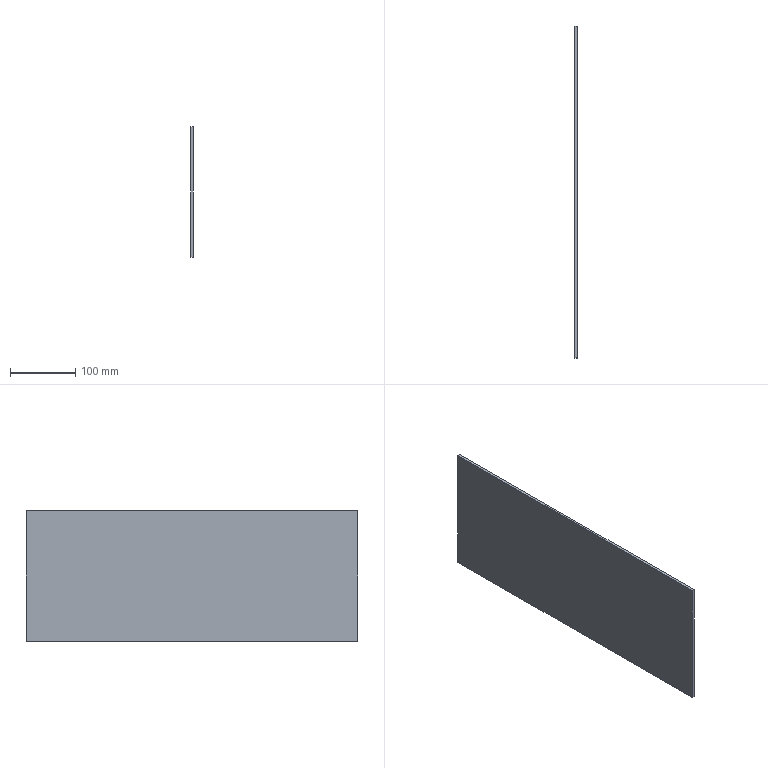Part | STEP file | 1 solid | 6 faces | box 4 x 509.4 x 200.9 mm | volume 409354 mm3 | plane 6
STEP:
#1=CARTESIAN_POINT('',(0.,0.,0.));
#2=DIRECTION('',(0.,0.,1.));
#3=DIRECTION('',(1.,0.,0.));
#4=AXIS2_PLACEMENT_3D('',#1,#2,#3);
#5=CARTESIAN_POINT('',(761.,3906.,1648.194));
#6=VERTEX_POINT('',#5);
#7=CARTESIAN_POINT('',(761.,3906.,1447.294));
#8=VERTEX_POINT('',#7);
#9=CARTESIAN_POINT('',(761.,3906.,1648.194));
#10=DIRECTION('',(0.,0.,-1.));
#11=VECTOR('',#10,1.);
#12=LINE('',#9,#11);
#13=CARTESIAN_POINT('',(765.,3906.,1447.294));
#14=DIRECTION('',(0.,-1.,0.));
#15=DIRECTION('',(0.,0.,-1.));
#16=AXIS2_PLACEMENT_3D('',#13,#14,#15);
#17=PLANE('',#16);
#18=CARTESIAN_POINT('',(-200.9,-4.));
#19=DIRECTION('',(1.,0.));
#20=VECTOR('',#19,1.);
#21=LINE('',#18,#20);
#22=(GEOMETRIC_REPRESENTATION_CONTEXT(2)PARAMETRIC_REPRESENTATION_CONTEXT()REPRESENTATION_CONTEXT('',''));
#23=DEFINITIONAL_REPRESENTATION('',(#21),#22);
#24=PCURVE('',#17,#23);
#25=CARTESIAN_POINT('',(761.,0.,0.));
#26=DIRECTION('',(-1.,0.,0.));
#27=DIRECTION('',(0.,0.,1.));
#28=AXIS2_PLACEMENT_3D('',#25,#26,#27);
#29=PLANE('',#28);
#30=CARTESIAN_POINT('',(1648.194,3906.));
#31=DIRECTION('',(-1.,0.));
#32=VECTOR('',#31,1.);
#33=LINE('',#30,#32);
#34=(GEOMETRIC_REPRESENTATION_CONTEXT(2)PARAMETRIC_REPRESENTATION_CONTEXT()REPRESENTATION_CONTEXT('',''));
#35=DEFINITIONAL_REPRESENTATION('',(#33),#34);
#36=PCURVE('',#29,#35);
#37=SURFACE_CURVE('',#12,(#24,#36),.PCURVE_S1.);
#38=EDGE_CURVE('',#6,#8,#37,.T.);
#39=ORIENTED_EDGE('',*,*,#38,.F.);
#40=CARTESIAN_POINT('',(765.,3906.,1648.194));
#41=VERTEX_POINT('',#40);
#42=CARTESIAN_POINT('',(761.,3906.,1648.194));
#43=DIRECTION('',(1.,0.,0.));
#44=VECTOR('',#43,1.);
#45=LINE('',#42,#44);
#46=CARTESIAN_POINT('',(-200.9,-4.));
#47=DIRECTION('',(0.,1.));
#48=VECTOR('',#47,1.);
#49=LINE('',#46,#48);
#50=(GEOMETRIC_REPRESENTATION_CONTEXT(2)PARAMETRIC_REPRESENTATION_CONTEXT()REPRESENTATION_CONTEXT('',''));
#51=DEFINITIONAL_REPRESENTATION('',(#49),#50);
#52=PCURVE('',#17,#51);
#53=CARTESIAN_POINT('',(765.,3906.,1648.194));
#54=DIRECTION('',(0.,0.,1.));
#55=DIRECTION('',(1.,0.,0.));
#56=AXIS2_PLACEMENT_3D('',#53,#54,#55);
#57=PLANE('',#56);
#58=CARTESIAN_POINT('',(-4.,0.));
#59=DIRECTION('',(1.,0.));
#60=VECTOR('',#59,1.);
#61=LINE('',#58,#60);
#62=(GEOMETRIC_REPRESENTATION_CONTEXT(2)PARAMETRIC_REPRESENTATION_CONTEXT()REPRESENTATION_CONTEXT('',''));
#63=DEFINITIONAL_REPRESENTATION('',(#61),#62);
#64=PCURVE('',#57,#63);
#65=SURFACE_CURVE('',#45,(#52,#64),.PCURVE_S1.);
#66=EDGE_CURVE('',#6,#41,#65,.T.);
#67=ORIENTED_EDGE('',*,*,#66,.T.);
#68=CARTESIAN_POINT('',(765.,3906.,1447.294));
#69=VERTEX_POINT('',#68);
#70=CARTESIAN_POINT('',(765.,3906.,1648.194));
#71=DIRECTION('',(0.,0.,-1.));
#72=VECTOR('',#71,1.);
#73=LINE('',#70,#72);
#74=CARTESIAN_POINT('',(-200.9,0.));
#75=DIRECTION('',(1.,0.));
#76=VECTOR('',#75,1.);
#77=LINE('',#74,#76);
#78=(GEOMETRIC_REPRESENTATION_CONTEXT(2)PARAMETRIC_REPRESENTATION_CONTEXT()REPRESENTATION_CONTEXT('',''));
#79=DEFINITIONAL_REPRESENTATION('',(#77),#78);
#80=PCURVE('',#17,#79);
#81=CARTESIAN_POINT('',(765.,0.,0.));
#82=DIRECTION('',(-1.,0.,0.));
#83=DIRECTION('',(0.,0.,1.));
#84=AXIS2_PLACEMENT_3D('',#81,#82,#83);
#85=PLANE('',#84);
#86=CARTESIAN_POINT('',(1648.194,3906.));
#87=DIRECTION('',(-1.,0.));
#88=VECTOR('',#87,1.);
#89=LINE('',#86,#88);
#90=(GEOMETRIC_REPRESENTATION_CONTEXT(2)PARAMETRIC_REPRESENTATION_CONTEXT()REPRESENTATION_CONTEXT('',''));
#91=DEFINITIONAL_REPRESENTATION('',(#89),#90);
#92=PCURVE('',#85,#91);
#93=SURFACE_CURVE('',#73,(#80,#92),.PCURVE_S1.);
#94=EDGE_CURVE('',#41,#69,#93,.T.);
#95=ORIENTED_EDGE('',*,*,#94,.T.);
#96=CARTESIAN_POINT('',(761.,3906.,1447.294));
#97=DIRECTION('',(1.,0.,0.));
#98=VECTOR('',#97,1.);
#99=LINE('',#96,#98);
#100=CARTESIAN_POINT('',(0.,-4.));
#101=DIRECTION('',(0.,1.));
#102=VECTOR('',#101,1.);
#103=LINE('',#100,#102);
#104=(GEOMETRIC_REPRESENTATION_CONTEXT(2)PARAMETRIC_REPRESENTATION_CONTEXT()REPRESENTATION_CONTEXT('',''));
#105=DEFINITIONAL_REPRESENTATION('',(#103),#104);
#106=PCURVE('',#17,#105);
#107=CARTESIAN_POINT('',(765.,4415.4,1447.294));
#108=DIRECTION('',(0.,0.,-1.));
#109=DIRECTION('',(0.,1.,0.));
#110=AXIS2_PLACEMENT_3D('',#107,#108,#109);
#111=PLANE('',#110);
#112=CARTESIAN_POINT('',(-509.4,-4.));
#113=DIRECTION('',(0.,1.));
#114=VECTOR('',#113,1.);
#115=LINE('',#112,#114);
#116=(GEOMETRIC_REPRESENTATION_CONTEXT(2)PARAMETRIC_REPRESENTATION_CONTEXT()REPRESENTATION_CONTEXT('',''));
#117=DEFINITIONAL_REPRESENTATION('',(#115),#116);
#118=PCURVE('',#111,#117);
#119=SURFACE_CURVE('',#99,(#106,#118),.PCURVE_S1.);
#120=EDGE_CURVE('',#8,#69,#119,.T.);
#121=ORIENTED_EDGE('',*,*,#120,.F.);
#122=EDGE_LOOP('',(#39,#67,#95,#121));
#123=FACE_BOUND('',#122,.F.);
#124=ADVANCED_FACE('',(#123),#17,.T.);
#125=ORIENTED_EDGE('',*,*,#38,.T.);
#126=CARTESIAN_POINT('',(761.,4415.4,1447.294));
#127=VERTEX_POINT('',#126);
#128=CARTESIAN_POINT('',(761.,3906.,1447.294));
#129=DIRECTION('',(0.,1.,0.));
#130=VECTOR('',#129,1.);
#131=LINE('',#128,#130);
#132=CARTESIAN_POINT('',(1447.294,3906.));
#133=DIRECTION('',(0.,1.));
#134=VECTOR('',#133,1.);
#135=LINE('',#132,#134);
#136=(GEOMETRIC_REPRESENTATION_CONTEXT(2)PARAMETRIC_REPRESENTATION_CONTEXT()REPRESENTATION_CONTEXT('',''));
#137=DEFINITIONAL_REPRESENTATION('',(#135),#136);
#138=PCURVE('',#29,#137);
#139=CARTESIAN_POINT('',(-509.4,-4.));
#140=DIRECTION('',(1.,0.));
#141=VECTOR('',#140,1.);
#142=LINE('',#139,#141);
#143=(GEOMETRIC_REPRESENTATION_CONTEXT(2)PARAMETRIC_REPRESENTATION_CONTEXT()REPRESENTATION_CONTEXT('',''));
#144=DEFINITIONAL_REPRESENTATION('',(#142),#143);
#145=PCURVE('',#111,#144);
#146=SURFACE_CURVE('',#131,(#138,#145),.PCURVE_S1.);
#147=EDGE_CURVE('',#8,#127,#146,.T.);
#148=ORIENTED_EDGE('',*,*,#147,.T.);
#149=CARTESIAN_POINT('',(761.,4415.4,1648.194));
#150=VERTEX_POINT('',#149);
#151=CARTESIAN_POINT('',(761.,4415.4,1447.294));
#152=DIRECTION('',(0.,0.,1.));
#153=VECTOR('',#152,1.);
#154=LINE('',#151,#153);
#155=CARTESIAN_POINT('',(1447.294,4415.4));
#156=DIRECTION('',(1.,0.));
#157=VECTOR('',#156,1.);
#158=LINE('',#155,#157);
#159=(GEOMETRIC_REPRESENTATION_CONTEXT(2)PARAMETRIC_REPRESENTATION_CONTEXT()REPRESENTATION_CONTEXT('',''));
#160=DEFINITIONAL_REPRESENTATION('',(#158),#159);
#161=PCURVE('',#29,#160);
#162=CARTESIAN_POINT('',(765.,4415.4,1648.194));
#163=DIRECTION('',(0.,1.,0.));
#164=DIRECTION('',(0.,0.,1.));
#165=AXIS2_PLACEMENT_3D('',#162,#163,#164);
#166=PLANE('',#165);
#167=CARTESIAN_POINT('',(-200.9,-4.));
#168=DIRECTION('',(1.,0.));
#169=VECTOR('',#168,1.);
#170=LINE('',#167,#169);
#171=(GEOMETRIC_REPRESENTATION_CONTEXT(2)PARAMETRIC_REPRESENTATION_CONTEXT()REPRESENTATION_CONTEXT('',''));
#172=DEFINITIONAL_REPRESENTATION('',(#170),#171);
#173=PCURVE('',#166,#172);
#174=SURFACE_CURVE('',#154,(#161,#173),.PCURVE_S1.);
#175=EDGE_CURVE('',#127,#150,#174,.T.);
#176=ORIENTED_EDGE('',*,*,#175,.T.);
#177=CARTESIAN_POINT('',(761.,4415.4,1648.194));
#178=DIRECTION('',(0.,-1.,0.));
#179=VECTOR('',#178,1.);
#180=LINE('',#177,#179);
#181=CARTESIAN_POINT('',(1648.194,4415.4));
#182=DIRECTION('',(0.,-1.));
#183=VECTOR('',#182,1.);
#184=LINE('',#181,#183);
#185=(GEOMETRIC_REPRESENTATION_CONTEXT(2)PARAMETRIC_REPRESENTATION_CONTEXT()REPRESENTATION_CONTEXT('',''));
#186=DEFINITIONAL_REPRESENTATION('',(#184),#185);
#187=PCURVE('',#29,#186);
#188=CARTESIAN_POINT('',(-4.,509.4));
#189=DIRECTION('',(0.,-1.));
#190=VECTOR('',#189,1.);
#191=LINE('',#188,#190);
#192=(GEOMETRIC_REPRESENTATION_CONTEXT(2)PARAMETRIC_REPRESENTATION_CONTEXT()REPRESENTATION_CONTEXT('',''));
#193=DEFINITIONAL_REPRESENTATION('',(#191),#192);
#194=PCURVE('',#57,#193);
#195=SURFACE_CURVE('',#180,(#187,#194),.PCURVE_S1.);
#196=EDGE_CURVE('',#150,#6,#195,.T.);
#197=ORIENTED_EDGE('',*,*,#196,.T.);
#198=EDGE_LOOP('',(#125,#148,#176,#197));
#199=FACE_BOUND('',#198,.F.);
#200=ADVANCED_FACE('',(#199),#29,.T.);
#201=ORIENTED_EDGE('',*,*,#147,.F.);
#202=ORIENTED_EDGE('',*,*,#120,.T.);
#203=CARTESIAN_POINT('',(765.,4415.4,1447.294));
#204=VERTEX_POINT('',#203);
#205=CARTESIAN_POINT('',(765.,3906.,1447.294));
#206=DIRECTION('',(0.,1.,0.));
#207=VECTOR('',#206,1.);
#208=LINE('',#205,#207);
#209=CARTESIAN_POINT('',(-509.4,0.));
#210=DIRECTION('',(1.,0.));
#211=VECTOR('',#210,1.);
#212=LINE('',#209,#211);
#213=(GEOMETRIC_REPRESENTATION_CONTEXT(2)PARAMETRIC_REPRESENTATION_CONTEXT()REPRESENTATION_CONTEXT('',''));
#214=DEFINITIONAL_REPRESENTATION('',(#212),#213);
#215=PCURVE('',#111,#214);
#216=CARTESIAN_POINT('',(1447.294,3906.));
#217=DIRECTION('',(0.,1.));
#218=VECTOR('',#217,1.);
#219=LINE('',#216,#218);
#220=(GEOMETRIC_REPRESENTATION_CONTEXT(2)PARAMETRIC_REPRESENTATION_CONTEXT()REPRESENTATION_CONTEXT('',''));
#221=DEFINITIONAL_REPRESENTATION('',(#219),#220);
#222=PCURVE('',#85,#221);
#223=SURFACE_CURVE('',#208,(#215,#222),.PCURVE_S1.);
#224=EDGE_CURVE('',#69,#204,#223,.T.);
#225=ORIENTED_EDGE('',*,*,#224,.T.);
#226=CARTESIAN_POINT('',(761.,4415.4,1447.294));
#227=DIRECTION('',(1.,0.,0.));
#228=VECTOR('',#227,1.);
#229=LINE('',#226,#228);
#230=CARTESIAN_POINT('',(0.,-4.));
#231=DIRECTION('',(0.,1.));
#232=VECTOR('',#231,1.);
#233=LINE('',#230,#232);
#234=(GEOMETRIC_REPRESENTATION_CONTEXT(2)PARAMETRIC_REPRESENTATION_CONTEXT()REPRESENTATION_CONTEXT('',''));
#235=DEFINITIONAL_REPRESENTATION('',(#233),#234);
#236=PCURVE('',#111,#235);
#237=CARTESIAN_POINT('',(-200.9,-4.));
#238=DIRECTION('',(0.,1.));
#239=VECTOR('',#238,1.);
#240=LINE('',#237,#239);
#241=(GEOMETRIC_REPRESENTATION_CONTEXT(2)PARAMETRIC_REPRESENTATION_CONTEXT()REPRESENTATION_CONTEXT('',''));
#242=DEFINITIONAL_REPRESENTATION('',(#240),#241);
#243=PCURVE('',#166,#242);
#244=SURFACE_CURVE('',#229,(#236,#243),.PCURVE_S1.);
#245=EDGE_CURVE('',#127,#204,#244,.T.);
#246=ORIENTED_EDGE('',*,*,#245,.F.);
#247=EDGE_LOOP('',(#201,#202,#225,#246));
#248=FACE_BOUND('',#247,.F.);
#249=ADVANCED_FACE('',(#248),#111,.T.);
#250=ORIENTED_EDGE('',*,*,#94,.F.);
#251=CARTESIAN_POINT('',(765.,4415.4,1648.194));
#252=VERTEX_POINT('',#251);
#253=CARTESIAN_POINT('',(765.,4415.4,1648.194));
#254=DIRECTION('',(0.,-1.,0.));
#255=VECTOR('',#254,1.);
#256=LINE('',#253,#255);
#257=CARTESIAN_POINT('',(1648.194,4415.4));
#258=DIRECTION('',(0.,-1.));
#259=VECTOR('',#258,1.);
#260=LINE('',#257,#259);
#261=(GEOMETRIC_REPRESENTATION_CONTEXT(2)PARAMETRIC_REPRESENTATION_CONTEXT()REPRESENTATION_CONTEXT('',''));
#262=DEFINITIONAL_REPRESENTATION('',(#260),#261);
#263=PCURVE('',#85,#262);
#264=CARTESIAN_POINT('',(0.,509.4));
#265=DIRECTION('',(0.,-1.));
#266=VECTOR('',#265,1.);
#267=LINE('',#264,#266);
#268=(GEOMETRIC_REPRESENTATION_CONTEXT(2)PARAMETRIC_REPRESENTATION_CONTEXT()REPRESENTATION_CONTEXT('',''));
#269=DEFINITIONAL_REPRESENTATION('',(#267),#268);
#270=PCURVE('',#57,#269);
#271=SURFACE_CURVE('',#256,(#263,#270),.PCURVE_S1.);
#272=EDGE_CURVE('',#252,#41,#271,.T.);
#273=ORIENTED_EDGE('',*,*,#272,.F.);
#274=CARTESIAN_POINT('',(765.,4415.4,1447.294));
#275=DIRECTION('',(0.,0.,1.));
#276=VECTOR('',#275,1.);
#277=LINE('',#274,#276);
#278=CARTESIAN_POINT('',(1447.294,4415.4));
#279=DIRECTION('',(1.,0.));
#280=VECTOR('',#279,1.);
#281=LINE('',#278,#280);
#282=(GEOMETRIC_REPRESENTATION_CONTEXT(2)PARAMETRIC_REPRESENTATION_CONTEXT()REPRESENTATION_CONTEXT('',''));
#283=DEFINITIONAL_REPRESENTATION('',(#281),#282);
#284=PCURVE('',#85,#283);
#285=CARTESIAN_POINT('',(-200.9,0.));
#286=DIRECTION('',(1.,0.));
#287=VECTOR('',#286,1.);
#288=LINE('',#285,#287);
#289=(GEOMETRIC_REPRESENTATION_CONTEXT(2)PARAMETRIC_REPRESENTATION_CONTEXT()REPRESENTATION_CONTEXT('',''));
#290=DEFINITIONAL_REPRESENTATION('',(#288),#289);
#291=PCURVE('',#166,#290);
#292=SURFACE_CURVE('',#277,(#284,#291),.PCURVE_S1.);
#293=EDGE_CURVE('',#204,#252,#292,.T.);
#294=ORIENTED_EDGE('',*,*,#293,.F.);
#295=ORIENTED_EDGE('',*,*,#224,.F.);
#296=EDGE_LOOP('',(#250,#273,#294,#295));
#297=FACE_BOUND('',#296,.F.);
#298=ADVANCED_FACE('',(#297),#85,.F.);
#299=ORIENTED_EDGE('',*,*,#196,.F.);
#300=CARTESIAN_POINT('',(761.,4415.4,1648.194));
#301=DIRECTION('',(1.,0.,0.));
#302=VECTOR('',#301,1.);
#303=LINE('',#300,#302);
#304=CARTESIAN_POINT('',(-4.,509.4));
#305=DIRECTION('',(1.,0.));
#306=VECTOR('',#305,1.);
#307=LINE('',#304,#306);
#308=(GEOMETRIC_REPRESENTATION_CONTEXT(2)PARAMETRIC_REPRESENTATION_CONTEXT()REPRESENTATION_CONTEXT('',''));
#309=DEFINITIONAL_REPRESENTATION('',(#307),#308);
#310=PCURVE('',#57,#309);
#311=CARTESIAN_POINT('',(0.,-4.));
#312=DIRECTION('',(0.,1.));
#313=VECTOR('',#312,1.);
#314=LINE('',#311,#313);
#315=(GEOMETRIC_REPRESENTATION_CONTEXT(2)PARAMETRIC_REPRESENTATION_CONTEXT()REPRESENTATION_CONTEXT('',''));
#316=DEFINITIONAL_REPRESENTATION('',(#314),#315);
#317=PCURVE('',#166,#316);
#318=SURFACE_CURVE('',#303,(#310,#317),.PCURVE_S1.);
#319=EDGE_CURVE('',#150,#252,#318,.T.);
#320=ORIENTED_EDGE('',*,*,#319,.T.);
#321=ORIENTED_EDGE('',*,*,#272,.T.);
#322=ORIENTED_EDGE('',*,*,#66,.F.);
#323=EDGE_LOOP('',(#299,#320,#321,#322));
#324=FACE_BOUND('',#323,.F.);
#325=ADVANCED_FACE('',(#324),#57,.T.);
#326=ORIENTED_EDGE('',*,*,#175,.F.);
#327=ORIENTED_EDGE('',*,*,#245,.T.);
#328=ORIENTED_EDGE('',*,*,#293,.T.);
#329=ORIENTED_EDGE('',*,*,#319,.F.);
#330=EDGE_LOOP('',(#326,#327,#328,#329));
#331=FACE_BOUND('',#330,.F.);
#332=ADVANCED_FACE('',(#331),#166,.T.);
#333=CLOSED_SHELL('',(#124,#200,#249,#298,#325,#332));
#334=MANIFOLD_SOLID_BREP('',#333);
#335=(LENGTH_UNIT()NAMED_UNIT(*)SI_UNIT(.MILLI.,.METRE.));
#336=UNCERTAINTY_MEASURE_WITH_UNIT(LENGTH_MEASURE(0.0000001),#335,'','');
#337=(NAMED_UNIT(*)PLANE_ANGLE_UNIT()SI_UNIT($,.RADIAN.));
#338=(NAMED_UNIT(*)SI_UNIT($,.STERADIAN.)SOLID_ANGLE_UNIT());
#339=(GEOMETRIC_REPRESENTATION_CONTEXT(3)GLOBAL_UNCERTAINTY_ASSIGNED_CONTEXT((#336))GLOBAL_UNIT_ASSIGNED_CONTEXT((#335,#337,#338))REPRESENTATION_CONTEXT('',''));
#340=ADVANCED_BREP_SHAPE_REPRESENTATION('',(#4,#334),#339);